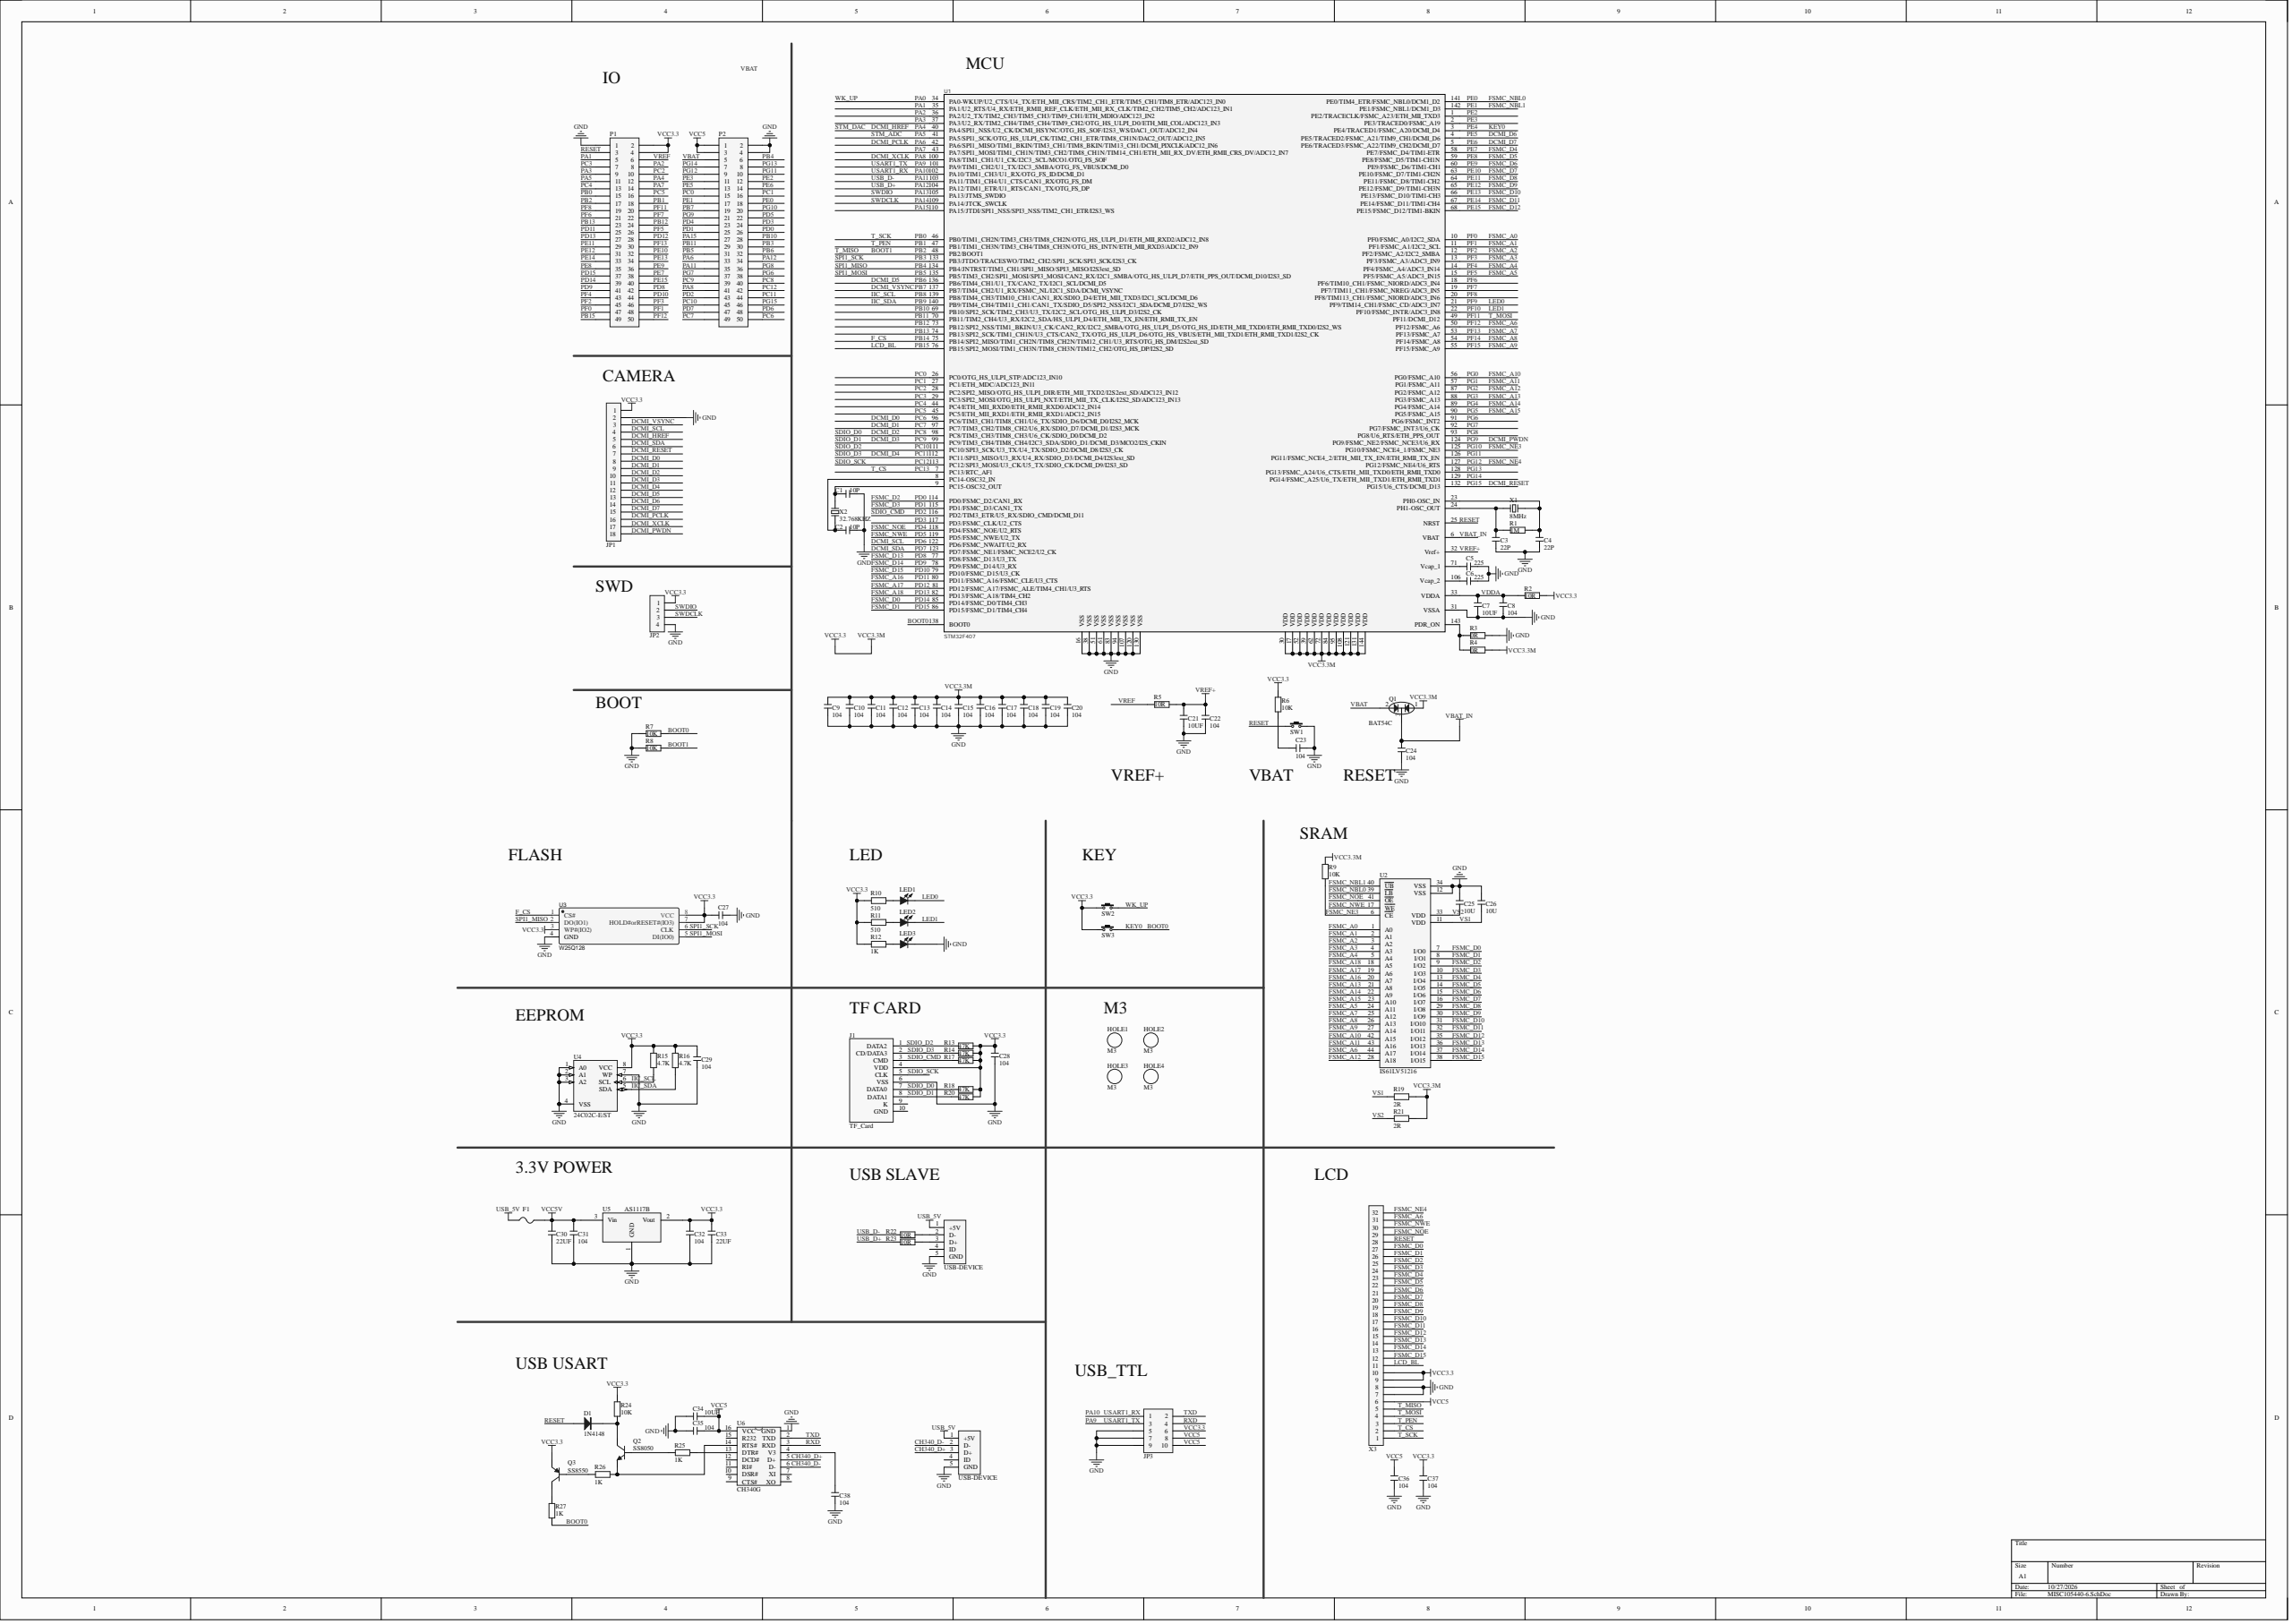Circuit board | Altium Designer | 97 parts | 148 nets
Bill of materials:
Comment,Description,Designator,Footprint,LibRef,Quantity
"10P","SMD capacitor","C1, C2","C 0402","C","2"
"22P","SMD capacitor","C3, C4","C 0402","C","2"
"225","SMD capacitor","C5, C6","C 0402","C","2"
"10UF","SMD capacitor","C7, C21, C34","C 0402","C","3"
"104","SMD capacitor, Non-polar SMD capacitor","C8, C9, C10, C11, C12, C13, C14, C15, C16, C17, C18, C19, C20, C22, C23, C24, C27, C28, C29, C31, C32, C35, C36, C37, C38","C 0402","C","25"
"10U","SMD capacitor","C25, C26","C 0402","C","2"
"22UF","SMD capacitor","C30, C33","C 0402","C","2"
"1N4148","Switching diode","D1","MINI_MELF (LL34)","1N4148","1"
"MSMD200-8V 2A","SMD fuse","F1","FU 0805","FU","1"
"M3","Copper pillar hole","HOLE1, HOLE2, HOLE3, HOLE4","M3 5.4MM","M3","4"
"TF_Card","TF card socket","J1","Micro SD","TF_Card","1"
"FPC0.5-18P","FPC connector","JP1","FPC0.5 2H-WS-18P","FPC-18P","1"
"SWD","4P connector","JP2","XH2.54-WI-4P","Header 4","1"
"Header 5X2","5*2P connector","JP3","HDR2.54-LI-2x5P","Header 5X2","1"
"Red","SMD LED","LED1, LED2, LED3","LED 0603R","LED-SMD","3"
"Header 25X2","Header, 25-Pin, Dual row","P1, P2","HDR2.54-LI-2x25P","Header 25X2","2"
"BAT54C","SMD Schottky diode","Q1","SOT23-3L","BAT54C","1"
"SS8050","RF amplifier, NPN type","Q2","SOT23-3L","8050-SMD","1"
"SS8550","RF amplifier, PNP type","Q3","SOT23-3L","8550-SMD","1"
"1M","SMD resistor","R1","R 0402","R","1"
"10R","SMD resistor","R2, R5, R22, R23","R 0402","R","4"
"0R","SMD resistor","R3, R4","R 0402","R","2"
"10K","SMD resistor","R6, R7, R8, R9, R24","R 0402","R","5"
"510","SMD resistor","R10, R11","R 0402","R","2"
"1K","SMD resistor","R12, R25, R26, R27","R 0402","R","4"
"47K","SMD resistor","R13, R14, R17, R18, R20","R 0402","R","5"
"4.7K","SMD resistor","R15, R16","R 0402","R","2"
"2R","SMD resistor","R19, R21","R 0402","R","2"
"3x6x5","3x6 tactile switch","SW1, SW2, SW3","TSW SMD-3*4*2.5","TSW 3x6","3"
"STM32F407","","U1","LQFP144 20X20_M","STM32F407","1"
"IS61LV51216","Static RAM","U2","TSOP44_M","IS61LV51216","1"
"W25Q128","","U3","SOP8W_L","W25Q128","1"
"24C02C-E/ST","2Kbit, 400kHz, 5V, I2C Serial EEPROM, 8-Pin TSSOP, Extended Temperature","U4","SOP8_L","24C02C-E/ST","1"
"AS1117B","Three-terminal voltage regulator","U5","SOT89_L","AMS1117","1"
"CH340G","USB2UART","U6","SOP16","CH340G","1"
"USB-DEVICE","Micro USB receptacle","USB1, USB2","USB-MICRO_B","USB-5P","2"
"8MHz","2-pin passive crystal oscillator","X1","OSC 5032-2P","XTAL-2P","1"
"32.768KHZ","2-pin passive crystal oscillator","X2","OSC 3215-2P","XTAL-2P","1"
"FPC0.5-32P","FPC connector","X3","FPC0.5 2H-WS-32P","FPC-32P","1"
Netlist (Protel format):
[
C1
C 0402
10P



]
[
C2
C 0402
10P



]
[
C3
C 0402
22P



]
[
C4
C 0402
22P



]
[
C5
C 0402
225



]
[
C6
C 0402
225



]
[
C7
C 0402
10UF



]
[
C8
C 0402
104



]
[
C9
C 0402
104



]
[
C10
C 0402
104



]
[
C11
C 0402
104



]
[
C12
C 0402
104



]
[
C13
C 0402
104



]
[
C14
C 0402
104



]
[
C15
C 0402
104



]
[
C16
C 0402
104



]
[
C17
C 0402
104



]
[
C18
C 0402
104



]
[
C19
C 0402
104



]
[
C20
C 0402
104



]
[
C21
C 0402
10UF



]
[
C22
C 0402
104



]
[
C23
C 0402
104



]
[
C24
C 0402
104



]
[
C25
C 0402
10U



]
[
C26
C 0402
10U



]
[
C27
C 0402
104



]
[
C28
C 0402
104



]
[
C29
C 0402
104



]
[
C30
C 0402
22UF



]
[
C31
C 0402
104



]
[
C32
C 0402
104



]
[
C33
C 0402
22UF



]
[
C34
C 0402
10UF



]
[
C35
C 0402
104



]
[
C36
C 0402
104



]
[
C37
C 0402
104



]
[
C38
C 0402
104



]
[
D1
MINI_MELF (LL34)
1N4148



]
[
F1
FU 0805
MSMD200-8V 2A



]
[
HOLE1
M3 5.4MM
M3



]
[
HOLE2
M3 5.4MM
M3



]
[
HOLE3
M3 5.4MM
M3



]
[
HOLE4
M3 5.4MM
M3



]
[
J1
Micro SD
TF_Card



]
[
JP1
FPC0.5 2H-WS-18P
FPC0.5-18P



]
[
JP2
XH2.54-WI-4P
SWD



]
[
JP3
HDR2.54-LI-2x5P
Header 5X2



]
[
LED1
LED 0603R
Red



]
[
LED2
LED 0603R
Red



]
[
LED3
LED 0603R
Red



]
[
P1
HDR2.54-LI-2x25P
Header 25X2



]
[
P2
HDR2.54-LI-2x25P
Header 25X2



]
[
Q1
SOT23-3L
BAT54C



]
[
Q2
SOT23-3L
SS8050



]
[
Q3
SOT23-3L
SS8550



]
[
R1
R 0402
1M



]
[
R2
R 0402
10R



]
[
R3
R 0402
0R



]
[
R4
R 0402
0R



]
[
R5
R 0402
10R



]
[
R6
R 0402
10K



]
[
R7
R 0402
10K



]
[
R8
R 0402
10K



]
[
R9
R 0402
10K



]
[
R10
R 0402
510



]
[
R11
R 0402
510



]
[
R12
R 0402
1K



]
[
R13
R 0402
47K



]
[
R14
R 0402
47K



]
[
R15
R 0402
4.7K



]
[
R16
R 0402
4.7K



]
[
R17
R 0402
47K



]
[
R18
R 0402
47K



]
[
R19
R 0402
2R



]
[
R20
R 0402
47K



]
[
R21
R 0402
2R



]
[
R22
R 0402
10R



]
[
R23
R 0402
10R



]
[
R24
R 0402
10K



]
[
R25
R 0402
1K



]
[
R26
R 0402
1K



]
[
R27
R 0402
1K



]
[
SW1
TSW SMD-3*4*2.5
3x6x5



]
[
SW2
TSW SMD-3*4*2.5
3x6x5



]
[
SW3
TSW SMD-3*4*2.5
3x6x5



]
[
U1
LQFP144 20X20_M
STM32F407



]
[
U2
TSOP44_M
IS61LV51216



]
[
U3
SOP8W_L
W25Q128



]
[
U4
SOP8_L
24C02C-E/ST



]
[
U5
SOT89_L
AS1117B



]
[
U6
SOP16
CH340G



]
[
USB1
USB-MICRO_B
USB-DEVICE



]
[
USB2
USB-MICRO_B
USB-DEVICE



]
[
X1
OSC 5032-2P
8MHz



]
[
X2
OSC 3215-2P
32.768KHZ



]
[
X3
FPC0.5 2H-WS-32P
FPC0.5-32P



]
(
VS2
C25-1
R21-2
U2-33
)
(
VS1
C26-1
R19-2
U2-11
)
(
VREF+
C21-1
C22-1
R5-2
U1-32
)
(
VREF
P1-6
R5-1
)
(
VDDA
C7-2
C8-2
R2-1
U1-33
)
(
VCC5V
C30-2
C31-2
F1-2
U5-3
)
(
VCC5
C34-1
C35-1
C36-2
JP3-8
JP3-10
P2-1
P2-3
U6-16
X3-6
)
(
VCC3.3
C9-2
C10-2
C11-2
C12-2
C13-2
C14-2
C15-2
C16-2
C17-2
C18-2
C19-2
C20-2
C27-1
C28-2
C29-2
C32-2
C33-2
C37-2
J1-4
JP1-1
JP2-1
JP3-6
P1-2
P1-4
Q1-1
Q3-2
R2-2
R4-2
R6-2
R9-2
R10-2
R11-2
R12-2
R13-1
R14-1
R15-2
R16-2
R17-1
R18-1
R19-1
R20-1
R21-1
R24-1
SW2-1
SW3-1
U1-17
U1-30
U1-39
U1-52
U1-62
U1-72
U1-84
U1-95
U1-108
U1-121
U1-131
U1-144
U3-3
U3-7
U3-8
U4-8
U5-2
X3-9
X3-10
)
(
VBAT_IN
C24-2
Q1-3
U1-6
)
(
VBAT
P2-5
Q1-2
)
(
USB_5V
F1-1
USB1-1
USB2-1
)
(
TXD
JP3-2
U6-2
)
(
RXD
JP3-4
U6-3
)
(
RESET
D1-1
P1-3
SW1-1
U1-25
X3-28
)
(
PG14
P2-7
U1-129
)
(
PG13
P2-8
U1-128
)
(
PG11
P2-10
U1-126
)
(
PG8
P2-36
U1-93
)
(
PG7
P2-37
U1-92
)
(
PG6
P2-38
U1-91
)
(
PF11
P1-20
U1-49
X3-4
)
(
PF8
P1-19
U1-20
)
(
PF7
P1-22
U1-19
)
(
PF6
P1-21
U1-18
)
(
PE3
P2-11
U1-2
)
(
PE2
P2-12
U1-1
)
(
PD3
P2-24
U1-117
)
(
PD2
J1-3
P2-43
R17-2
U1-116
)
(
PC13
U1-7
X3-2
)
(
PC12
J1-5
P2-42
U1-113
)
(
PC10
P2-45
U1-111
)
(
PC5
P1-16
U1-45
)
(
PC4
P1-13
U1-44
)
(
PC3
P1-7
U1-29
)
(
PC2
P1-10
U1-28
)
(
PC1
P2-16
U1-27
)
(
PC0
P2-15
U1-26
)
(
PB13
P1-23
U1-74
)
(
PB12
P1-24
U1-73
)
(
PB11
P2-29
U1-70
)
(
PB10
P2-28
U1-69
)
(
PB5
P2-31
U1-135
U3-5
)
(
PB4
P2-6
U1-134
U3-2
)
(
PB3
P2-30
U1-133
U3-6
)
(
PB1
P1-18
U1-47
X3-3
)
(
PB0
P1-15
U1-46
X3-1
)
(
PA15
P2-27
U1-110
)
(
PA14
JP2-3
U1-109
)
(
PA13
JP2-2
U1-105
)
(
PA12
P2-34
R23-2
U1-104
)
(
PA11
P2-35
R22-2
U1-103
)
(
PA10
JP3-1
U1-102
)
(
PA9
JP3-3
U1-101
)
(
PA7
P1-14
U1-43
)
(
PA5
P1-11
U1-41
)
(
PA3
P1-9
U1-37
)
(
PA2
P1-8
U1-36
)
(
PA1
P1-5
U1-35
)
(
PA0
SW2-2
U1-34
)
(
NetR25_1
R25-1
U6-13
)
(
NetR23_1
R23-1
USB1-3
)
(
NetR22_1
R22-1
USB1-2
)
(
NetR3_1
R3-1
R4-1
U1-143
)
(
NetQ3_3
Q3-3
R27-1
)
(
NetQ3_1
Q3-1
R26-2
)
(
NetQ2_2
Q2-2
R26-1
U6-14
)
(
NetQ2_1
Q2-1
R25-2
)
(
NetLED3_1
LED3-1
R12-1
)
(
NetLED2_1
LED2-1
R11-1
)
(
NetLED1_1
LED1-1
R10-1
)
(
NetJ1_1
J1-1
R13-2
)
(
NetD1_2
D1-2
Q2-3
R24-2
)
(
NetC38_2
C38-2
U6-4
)
(
NetC23_1
C23-1
R6-1
)
(
NetC6_1
C6-1
U1-106
)
(
NetC5_1
C5-1
U1-71
)
(
NetC4_2
C4-2
R1-2
U1-23
X1-2
)
(
NetC3_2
C3-2
R1-1
U1-24
X1-1
)
(
NetC2_2
C2-2
U1-8
X2-1
)
(
NetC1_2
C1-2
U1-9
X2-2
)
(
LED1
LED2-2
U1-22
)
(
LED0
LED1-2
U1-21
)
(
LCD_BL
P1-49
U1-76
X3-11
)
(
IIC_SDA
R16-1
U1-140
U4-5
)
(
IIC_SCL
R15-1
U1-139
U4-6
)
(
GND
C1-1
C2-1
C3-1
C4-1
C5-2
C6-2
C7-1
C8-1
C9-1
C10-1
C11-1
C12-1
C13-1
C14-1
C15-1
C16-1
C17-1
C18-1
C19-1
C20-1
C21-2
C22-2
C23-2
C24-1
C25-2
C26-2
C27-2
C28-1
C29-1
C30-1
C31-1
C32-1
C33-1
C34-2
C35-2
C36-1
C37-1
C38-1
J1-6
JP1-2
JP2-4
JP3-5
JP3-7
JP3-9
LED3-2
P1-1
P2-2
P2-4
R3-2
R7-1
R8-1
SW1-2
U1-16
U1-31
U1-38
U1-51
U1-61
U1-83
U1-94
U1-107
U1-120
U1-130
U2-12
U2-34
U3-4
U4-1
U4-2
U4-3
U4-4
U4-7
U5-1
U6-1
USB1-5
USB2-5
X3-7
X3-8
)
(
FSMC_NWE
P2-22
U1-119
U2-17
X3-30
)
(
FSMC_NOE
P2-23
U1-118
U2-41
X3-29
)
(
FSMC_NE4
P2-9
U1-127
X3-32
)
(
FSMC_NE3
P2-20
R9-1
U1-125
U2-6
)
(
FSMC_NBL1
P2-17
U1-142
U2-40
)
(
FSMC_NBL0
P2-18
U1-141
U2-39
)
(
FSMC_D15
P1-44
U1-79
U2-38
X3-12
)
(
FSMC_D14
P1-41
U1-78
U2-37
X3-13
)
(
FSMC_D13
P1-42
U1-77
U2-36
X3-14
)
(
FSMC_D12
P1-40
U1-68
U2-35
X3-15
)
(
FSMC_D11
P1-33
U1-67
U2-32
X3-16
)
(
FSMC_D10
P1-34
U1-66
U2-31
X3-17
)
(
FSMC_D9
P1-31
U1-65
U2-30
X3-18
)
(
FSMC_D8
P1-29
U1-64
U2-29
X3-19
)
(
FSMC_D7
P1-32
U1-63
U2-16
X3-20
)
(
FSMC_D6
P1-36
U1-60
U2-15
X3-21
)
(
FSMC_D5
P1-35
U1-59
U2-14
X3-22
)
(
FSMC_D4
P1-38
U1-58
U2-13
X3-23
)
(
FSMC_D3
P2-25
U1-115
U2-10
X3-24
)
(
FSMC_D2
P2-26
U1-114
U2-9
X3-25
)
(
FSMC_D1
P1-37
U1-86
U2-8
X3-26
)
(
FSMC_D0
P1-39
U1-85
U2-7
X3-27
)
(
FSMC_A18
P1-27
U1-82
U2-18
)
(
FSMC_A17
P1-28
U1-81
U2-19
)
(
FSMC_A16
P1-25
U1-80
U2-20
)
(
FSMC_A15
U1-90
U2-23
)
(
FSMC_A14
U1-89
U2-22
)
(
FSMC_A13
U1-88
U2-21
)
(
FSMC_A12
U1-87
U2-28
)
(
FSMC_A11
U1-57
U2-43
)
(
FSMC_A10
U1-56
U2-42
)
(
FSMC_A9
U1-55
U2-27
)
(
FSMC_A8
U1-54
U2-26
)
(
FSMC_A7
P1-30
U1-53
U2-25
)
(
FSMC_A6
P1-50
U1-50
U2-44
X3-31
)
(
FSMC_A5
P1-26
U1-15
U2-24
)
(
FSMC_A4
P1-43
U1-14
U2-5
)
(
FSMC_A3
P1-46
U1-13
U2-4
)
(
FSMC_A2
P1-45
U1-12
U2-3
)
(
FSMC_A1
P1-48
U1-11
U2-2
)
(
FSMC_A0
P1-47
U1-10
U2-1
)
(
F_CS
U1-75
U3-1
)
(
DCMI_XCLK
JP1-17
P2-41
U1-100
)
(
DCMI_VSYNC
JP1-3
P2-19
U1-137
)
(
DCMI_SDA
JP1-6
P2-47
U1-123
)
(
DCMI_SCL
JP1-4
P2-48
U1-122
)
(
DCMI_RESET
JP1-7
P2-46
U1-132
)
(
DCMI_PWDN
JP1-18
P2-21
U1-124
)
(
DCMI_PCLK
JP1-16
P2-33
U1-42
)
(
DCMI_HREF
JP1-5
P1-12
U1-40
)
(
DCMI_D7
JP1-15
P2-14
U1-5
)
(
DCMI_D6
JP1-14
P2-13
U1-4
)
(
DCMI_D5
JP1-13
P2-32
U1-136
)
(
DCMI_D4
J1-2
JP1-12
P2-44
R14-2
U1-112
)
(
DCMI_D3
J1-8
JP1-11
P2-39
R20-2
U1-99
)
(
DCMI_D2
J1-7
JP1-10
P2-40
R18-2
U1-98
)
(
DCMI_D1
JP1-9
P2-49
U1-97
)
(
DCMI_D0
JP1-8
P2-50
U1-96
)
(
CH340_D-
U6-6
USB2-2
)
(
CH340_D+
U6-5
USB2-3
)
(
BOOT1
P1-17
R8-2
U1-48
X3-5
)
(
BOOT0
R7-2
R27-2
SW3-2
U1-3
U1-138
)